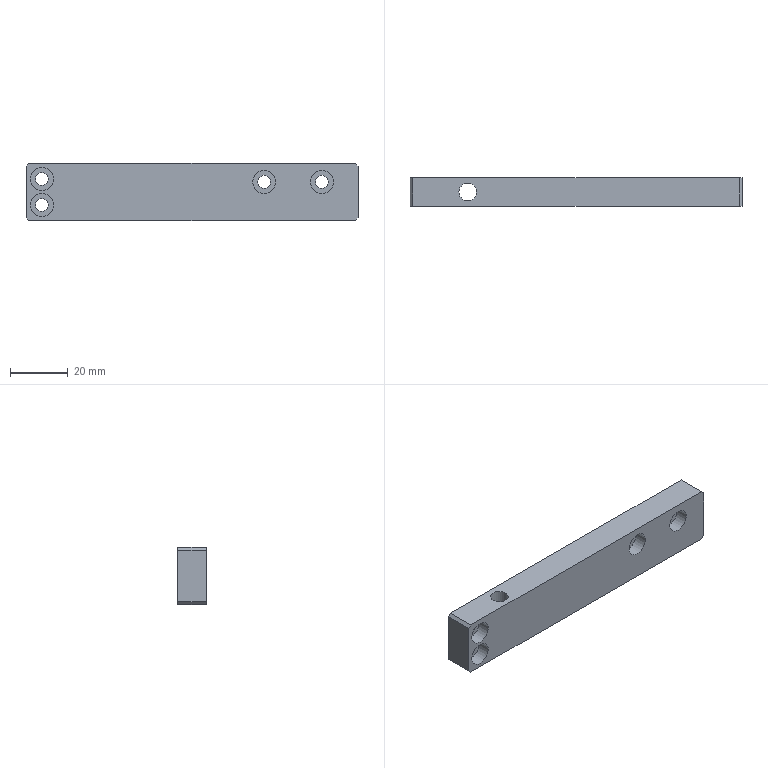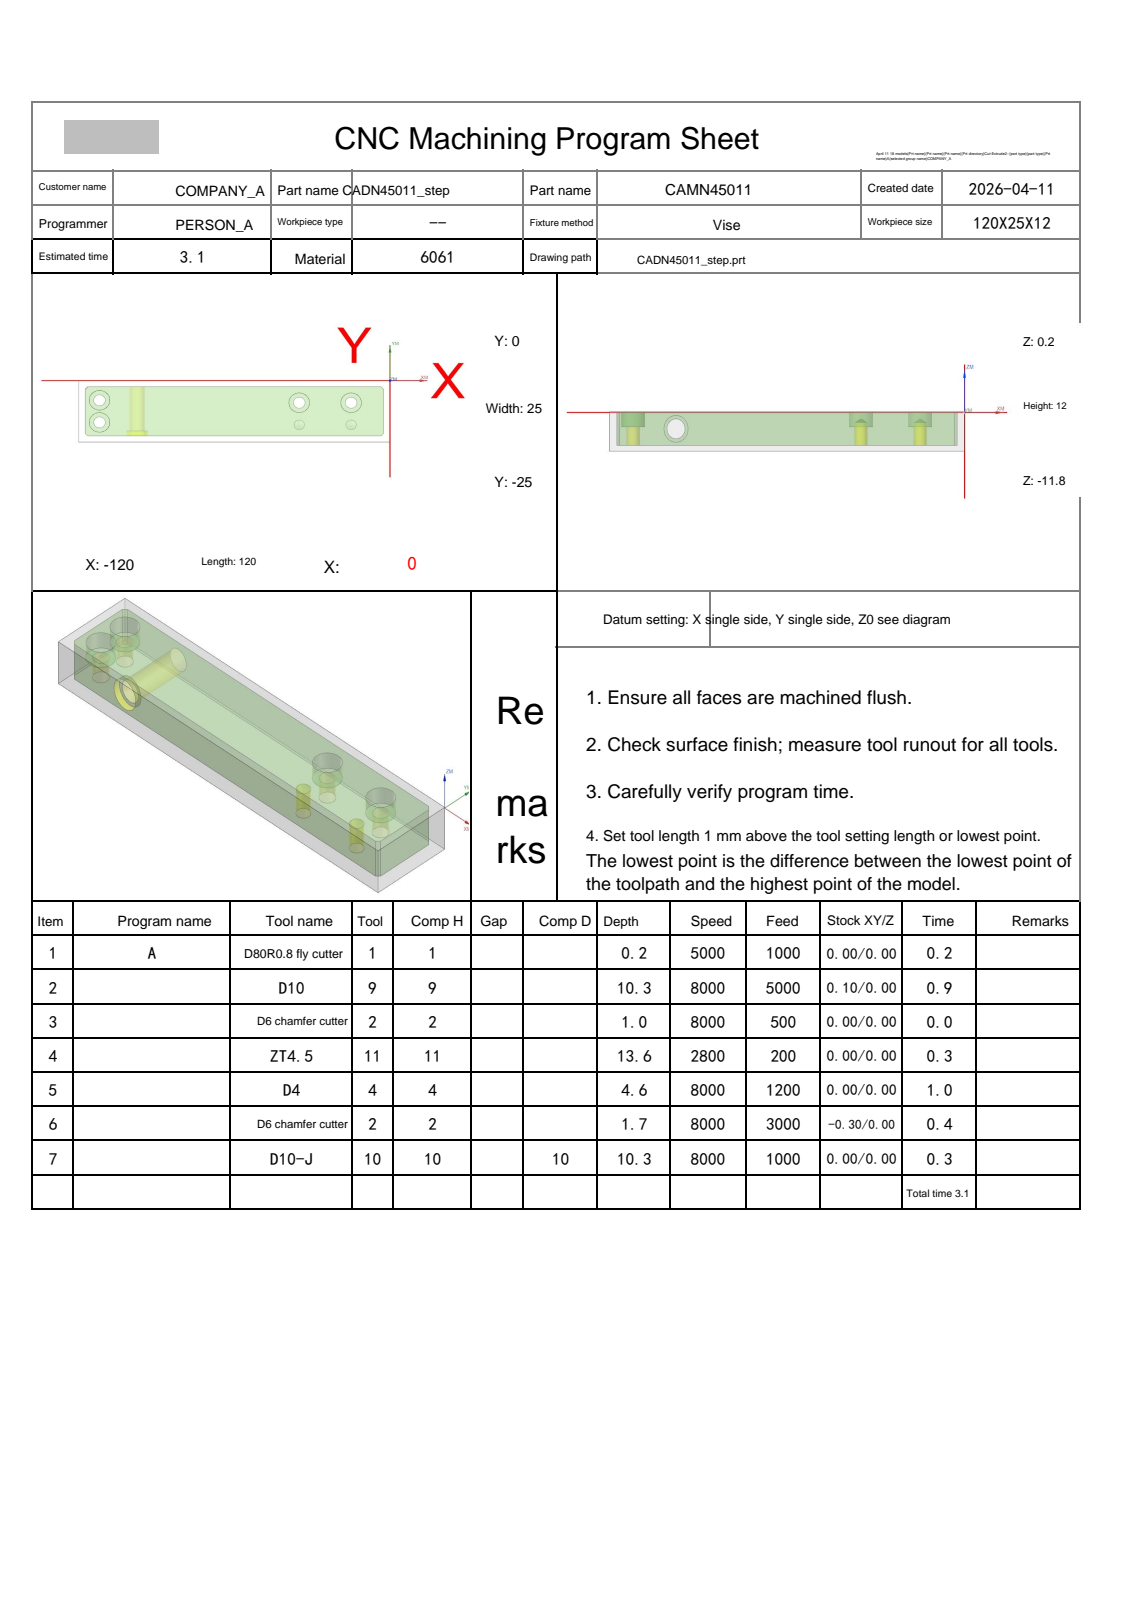NC program | NX | posted by the shop | part box 115 x 10 x 20 mm
Whole program:
%
O0001
(Machine time: 4.57 MIN)
(===Total Tool:6===)
(T1=D80R0.8 fly cutter D=80.  R=0.8  D-  H01 Z=0.    )
(T9=D10     D=10.  R=0.   D-  H09 Z=-10.1 )
(T2=D6 chamfer cutter   D=6.   R=0.   D-  H02 Z=-1.5  )
(T11=ZT4.5  D=4.5  DR_a=118 D-  H11 Z=-13.35)
(T4=D4      D=4.   R=0.   D4  H04 Z=-4.4  )
(T10=D10-J  D=10.  R=0.   D10 H10 Z=-10.1 )
G80 G90 G17 G49 G40
G91 G28 Z0
M01
N1 T01 M06
(D80R0.8 fly cutter  D=80. R=0.8 H=01 ce=0.00 di=0.00)
G00 G90 G54 X42.5 Y-12.5 M03 S5000
G43 H01 Z20.
M08
Z2.
G01 Z0.0 F1000.
X37.5
X-157.5
X-162.5
Z2.
G00 Z20.
G91 G28 Z0.0
M05
M09
G91 G28 Z0.0
M01
N2 T09 M06
(D10  D=10. R=0. H=09 ce=0.10 di=0.00)
G00 G90 G54 X-60. Y2.6 M03 S8000
G43 H09 Z20.
M08
Z.5
G01 X-3.5 Z.357 F5000.
G02 X.106 Y1.106 Z.347 I0.0 J-5.1
G01 X1.106 Y.106 Z.344
G02 X2.6 Y-3.5 Z.333 I-3.606 J-3.606
G01 Y-21.5 Z.288
G02 X1.106 Y-25.106 Z.278 I-5.1 J0.0
G01 X.106 Y-26.106 Z.274
G02 X-3.5 Y-27.6 Z.264 I-3.606 J3.606
G01 X-116.5 Z-.021
G02 X-120.106 Y-26.106 Z-.031 I0.0 J5.1
G01 X-121.106 Y-25.106 Z-.035
G02 X-122.6 Y-21.5 Z-.045 I3.606 J3.606
G01 Y-3.5 Z-.091
G02 X-121.106 Y.106 Z-.101 I5.1 J0.0
G01 X-120.106 Y1.106 Z-.104
G02 X-116.5 Y2.6 Z-.114 I3.606 J-3.606
G01 X-3.5 Z-.4
G02 X.106 Y1.106 Z-.41 I0.0 J-5.1
G01 X1.106 Y.106 Z-.414
G02 X2.6 Y-3.5 Z-.424 I-3.606 J-3.606
G01 Y-21.5 Z-.469
G02 X1.106 Y-25.106 Z-.479 I-5.1 J0.0
G01 X.106 Y-26.106 Z-.483
G02 X-3.5 Y-27.6 Z-.493 I-3.606 J3.606
G01 X-116.5 Z-.778
G02 X-120.106 Y-26.106 Z-.789 I0.0 J5.1
G01 X-121.106 Y-25.106 Z-.792
G02 X-122.6 Y-21.5 Z-.802 I3.606 J3.606
G01 Y-3.5 Z-.848
G02 X-121.106 Y.106 Z-.858 I5.1 J0.0
G01 X-120.106 Y1.106 Z-.861
G02 X-116.5 Y2.6 Z-.872 I3.606 J-3.606
G01 X-3.5 Z-1.157
G02 X.106 Y1.106 Z-1.167 I0.0 J-5.1
G01 X1.106 Y.106 Z-1.171
G02 X2.6 Y-3.5 Z-1.181 I-3.606 J-3.606
G01 Y-21.5 Z-1.226
G02 X1.106 Y-25.106 Z-1.236 I-5.1 J0.0
G01 X.106 Y-26.106 Z-1.24
G02 X-3.5 Y-27.6 Z-1.25 I-3.606 J3.606
G01 X-116.5 Z-1.536
G02 X-120.106 Y-26.106 Z-1.546 I0.0 J5.1
G01 X-121.106 Y-25.106 Z-1.549
G02 X-122.6 Y-21.5 Z-1.559 I3.606 J3.606
G01 Y-3.5 Z-1.605
G02 X-121.106 Y.106 Z-1.615 I5.1 J0.0
G01 X-120.106 Y1.106 Z-1.619
G02 X-116.5 Y2.6 Z-1.629 I3.606 J-3.606
G01 X-3.5 Z-1.914
G02 X.106 Y1.106 Z-1.924 I0.0 J-5.1
G01 X1.106 Y.106 Z-1.928
G02 X2.6 Y-3.5 Z-1.938 I-3.606 J-3.606
G01 Y-21.5 Z-1.983
G02 X1.106 Y-25.106 Z-1.994 I-5.1 J0.0
G01 X.106 Y-26.106 Z-1.997
G02 X-3.5 Y-27.6 Z-2.007 I-3.606 J3.606
G01 X-116.5 Z-2.293
G02 X-120.106 Y-26.106 Z-2.303 I0.0 J5.1
G01 X-121.106 Y-25.106 Z-2.306
G02 X-122.6 Y-21.5 Z-2.317 I3.606 J3.606
G01 Y-3.5 Z-2.362
G02 X-121.106 Y.106 Z-2.372 I5.1 J0.0
G01 X-120.106 Y1.106 Z-2.376
G02 X-116.5 Y2.6 Z-2.386 I3.606 J-3.606
G01 X-3.5 Z-2.671
G02 X.106 Y1.106 Z-2.681 I0.0 J-5.1
G01 X1.106 Y.106 Z-2.685
G02 X2.6 Y-3.5 Z-2.695 I-3.606 J-3.606
G01 Y-21.5 Z-2.741
G02 X1.106 Y-25.106 Z-2.751 I-5.1 J0.0
G01 X.106 Y-26.106 Z-2.754
G02 X-3.5 Y-27.6 Z-2.764 I-3.606 J3.606
G01 X-116.5 Z-3.05
G02 X-120.106 Y-26.106 Z-3.06 I0.0 J5.1
G01 X-121.106 Y-25.106 Z-3.064
G02 X-122.6 Y-21.5 Z-3.074 I3.606 J3.606
G01 Y-3.5 Z-3.119
G02 X-121.106 Y.106 Z-3.129 I5.1 J0.0
G01 X-120.106 Y1.106 Z-3.133
G02 X-116.5 Y2.6 Z-3.143 I3.606 J-3.606
G01 X-3.5 Z-3.428
G02 X.106 Y1.106 Z-3.439 I0.0 J-5.1
G01 X1.106 Y.106 Z-3.442
G02 X2.6 Y-3.5 Z-3.452 I-3.606 J-3.606
G01 Y-21.5 Z-3.498
G02 X1.106 Y-25.106 Z-3.508 I-5.1 J0.0
G01 X.106 Y-26.106 Z-3.511
G02 X-3.5 Y-27.6 Z-3.522 I-3.606 J3.606
G01 X-116.5 Z-3.807
G02 X-120.106 Y-26.106 Z-3.817 I0.0 J5.1
G01 X-121.106 Y-25.106 Z-3.821
G02 X-122.6 Y-21.5 Z-3.831 I3.606 J3.606
G01 Y-3.5 Z-3.876
G02 X-121.106 Y.106 Z-3.886 I5.1 J0.0
G01 X-120.106 Y1.106 Z-3.89
G02 X-116.5 Y2.6 Z-3.9 I3.606 J-3.606
G01 X-3.5 Z-4.186
G02 X.106 Y1.106 Z-4.196 I0.0 J-5.1
G01 X1.106 Y.106 Z-4.199
G02 X2.6 Y-3.5 Z-4.209 I-3.606 J-3.606
G01 Y-21.5 Z-4.255
G02 X1.106 Y-25.106 Z-4.265 I-5.1 J0.0
G01 X.106 Y-26.106 Z-4.269
G02 X-3.5 Y-27.6 Z-4.279 I-3.606 J3.606
G01 X-116.5 Z-4.564
G02 X-120.106 Y-26.106 Z-4.574 I0.0 J5.1
G01 X-121.106 Y-25.106 Z-4.578
G02 X-122.6 Y-21.5 Z-4.588 I3.606 J3.606
G01 Y-3.5 Z-4.633
G02 X-121.106 Y.106 Z-4.644 I5.1 J0.0
G01 X-120.106 Y1.106 Z-4.647
G02 X-116.5 Y2.6 Z-4.657 I3.606 J-3.606
G01 X-3.5 Z-4.943
G02 X.106 Y1.106 Z-4.953 I0.0 J-5.1
G01 X1.106 Y.106 Z-4.956
G02 X2.6 Y-3.5 Z-4.967 I-3.606 J-3.606
G01 Y-21.5 Z-5.012
G02 X1.106 Y-25.106 Z-5.022 I-5.1 J0.0
G01 X.106 Y-26.106 Z-5.026
G02 X-3.5 Y-27.6 Z-5.036 I-3.606 J3.606
G01 X-116.5 Z-5.321
G02 X-120.106 Y-26.106 Z-5.331 I0.0 J5.1
G01 X-121.106 Y-25.106 Z-5.335
G02 X-122.6 Y-21.5 Z-5.345 I3.606 J3.606
G01 Y-3.5 Z-5.391
G02 X-121.106 Y.106 Z-5.401 I5.1 J0.0
G01 X-120.106 Y1.106 Z-5.404
G02 X-116.5 Y2.6 Z-5.414 I3.606 J-3.606
G01 X-3.5 Z-5.7
G02 X.106 Y1.106 Z-5.71 I0.0 J-5.1
G01 X1.106 Y.106 Z-5.714
G02 X2.6 Y-3.5 Z-5.724 I-3.606 J-3.606
G01 Y-21.5 Z-5.769
G02 X1.106 Y-25.106 Z-5.779 I-5.1 J0.0
G01 X.106 Y-26.106 Z-5.783
G02 X-3.5 Y-27.6 Z-5.793 I-3.606 J3.606
G01 X-116.5 Z-6.078
G02 X-120.106 Y-26.106 Z-6.089 I0.0 J5.1
G01 X-121.106 Y-25.106 Z-6.092
G02 X-122.6 Y-21.5 Z-6.102 I3.606 J3.606
G01 Y-3.5 Z-6.148
G02 X-121.106 Y.106 Z-6.158 I5.1 J0.0
G01 X-120.106 Y1.106 Z-6.161
G02 X-116.5 Y2.6 Z-6.172 I3.606 J-3.606
G01 X-3.5 Z-6.457
G02 X.106 Y1.106 Z-6.467 I0.0 J-5.1
G01 X1.106 Y.106 Z-6.471
G02 X2.6 Y-3.5 Z-6.481 I-3.606 J-3.606
G01 Y-21.5 Z-6.526
G02 X1.106 Y-25.106 Z-6.536 I-5.1 J0.0
G01 X.106 Y-26.106 Z-6.54
G02 X-3.5 Y-27.6 Z-6.55 I-3.606 J3.606
G01 X-116.5 Z-6.836
G02 X-120.106 Y-26.106 Z-6.846 I0.0 J5.1
G01 X-121.106 Y-25.106 Z-6.849
G02 X-122.6 Y-21.5 Z-6.859 I3.606 J3.606
G01 Y-3.5 Z-6.905
G02 X-121.106 Y.106 Z-6.915 I5.1 J0.0
G01 X-120.106 Y1.106 Z-6.919
G02 X-116.5 Y2.6 Z-6.929 I3.606 J-3.606
G01 X-3.5 Z-7.214
G02 X.106 Y1.106 Z-7.224 I0.0 J-5.1
G01 X1.106 Y.106 Z-7.228
G02 X2.6 Y-3.5 Z-7.238 I-3.606 J-3.606
G01 Y-21.5 Z-7.283
G02 X1.106 Y-25.106 Z-7.294 I-5.1 J0.0
G01 X.106 Y-26.106 Z-7.297
G02 X-3.5 Y-27.6 Z-7.307 I-3.606 J3.606
G01 X-116.5 Z-7.593
G02 X-120.106 Y-26.106 Z-7.603 I0.0 J5.1
G01 X-121.106 Y-25.106 Z-7.606
G02 X-122.6 Y-21.5 Z-7.617 I3.606 J3.606
G01 Y-3.5 Z-7.662
G02 X-121.106 Y.106 Z-7.672 I5.1 J0.0
G01 X-120.106 Y1.106 Z-7.676
G02 X-116.5 Y2.6 Z-7.686 I3.606 J-3.606
G01 X-3.5 Z-7.971
G02 X.106 Y1.106 Z-7.981 I0.0 J-5.1
G01 X1.106 Y.106 Z-7.985
G02 X2.6 Y-3.5 Z-7.995 I-3.606 J-3.606
G01 Y-21.5 Z-8.041
G02 X1.106 Y-25.106 Z-8.051 I-5.1 J0.0
G01 X.106 Y-26.106 Z-8.054
G02 X-3.5 Y-27.6 Z-8.064 I-3.606 J3.606
G01 X-116.5 Z-8.35
G02 X-120.106 Y-26.106 Z-8.36 I0.0 J5.1
G01 X-121.106 Y-25.106 Z-8.364
G02 X-122.6 Y-21.5 Z-8.374 I3.606 J3.606
G01 Y-3.5 Z-8.419
G02 X-121.106 Y.106 Z-8.429 I5.1 J0.0
G01 X-120.106 Y1.106 Z-8.433
G02 X-116.5 Y2.6 Z-8.443 I3.606 J-3.606
G01 X-3.5 Z-8.728
G02 X.106 Y1.106 Z-8.739 I0.0 J-5.1
G01 X1.106 Y.106 Z-8.742
G02 X2.6 Y-3.5 Z-8.752 I-3.606 J-3.606
G01 Y-21.5 Z-8.798
G02 X1.106 Y-25.106 Z-8.808 I-5.1 J0.0
G01 X.106 Y-26.106 Z-8.811
G02 X-3.5 Y-27.6 Z-8.822 I-3.606 J3.606
G01 X-116.5 Z-9.107
G02 X-120.106 Y-26.106 Z-9.117 I0.0 J5.1
G01 X-121.106 Y-25.106 Z-9.121
G02 X-122.6 Y-21.5 Z-9.131 I3.606 J3.606
G01 Y-3.5 Z-9.176
G02 X-121.106 Y.106 Z-9.186 I5.1 J0.0
G01 X-120.106 Y1.106 Z-9.19
G02 X-116.5 Y2.6 Z-9.2 I3.606 J-3.606
G01 X-3.5 Z-9.486
G02 X.106 Y1.106 Z-9.496 I0.0 J-5.1
G01 X1.106 Y.106 Z-9.499
G02 X2.6 Y-3.5 Z-9.509 I-3.606 J-3.606
G01 Y-21.5 Z-9.555
G02 X1.106 Y-25.106 Z-9.565 I-5.1 J0.0
G01 X.106 Y-26.106 Z-9.569
G02 X-3.5 Y-27.6 Z-9.579 I-3.606 J3.606
G01 X-116.5 Z-9.864
G02 X-120.106 Y-26.106 Z-9.874 I0.0 J5.1
G01 X-121.106 Y-25.106 Z-9.878
G02 X-122.6 Y-21.5 Z-9.888 I3.606 J3.606
G01 Y-3.5 Z-9.933
G02 X-121.106 Y.106 Z-9.944 I5.1 J0.0
G01 X-120.106 Y1.106 Z-9.947
G02 X-116.5 Y2.6 Z-9.957 I3.606 J-3.606
G01 X-60. Z-10.1
X-3.5
G02 X.106 Y1.106 I0.0 J-5.1
G01 X1.106 Y.106
G02 X2.6 Y-3.5 I-3.606 J-3.606
G01 Y-21.5
G02 X1.106 Y-25.106 I-5.1 J0.0
G01 X.106 Y-26.106
G02 X-3.5 Y-27.6 I-3.606 J3.606
G01 X-116.5
G02 X-120.106 Y-26.106 I0.0 J5.1
G01 X-121.106 Y-25.106
G02 X-122.6 Y-21.5 I3.606 J3.606
G01 Y-3.5
G02 X-121.106 Y.106 I5.1 J0.0
G01 X-120.106 Y1.106
G02 X-116.5 Y2.6 I3.606 J-3.606
G01 X-60.
X-59.5
Z-9.1
G00 Z20.
G91 G28 Z0.0
M05
M09
G91 G28 Z0.0
M01
N3 T02 M06
(D6 chamfer cutter  D=6. R=0. H=02 ce=0.00 di=0.00)
G00 G90 G54 X-112. Y-17. M03 S8000
G43 H02 Z20.
M08
G98 G81 X-112. Y-17. Z-.8 R1. F500.
Y-8.
X-35. Y-9.
X-15.
G80
G00 Z20.
G91 G28 Z0.0
M05
M09
G91 G28 Z0.0
M01
N4 T11 M06
(ZT4.5 D=4.5 DR_a=118 H=11)
G00 G90 G54 X-112. Y-17. M03 S2800
G43 H11 Z20.
M08
G98 G83 X-112. Y-17. Z-13.352 R1. F200. Q2.
Y-8.
X-35. Y-9.
X-15.
G80
G00 Z20.
G91 G28 Z0.0
M05
M09
G91 G28 Z0.0
M01
N5 T04 M06
(D4  D=4. R=0. H=04 ce=0.10 di=0.00)
G00 G90 G54 X-112. Y-8. M03 S8000
G43 H04 Z20.
M08
Z.5
G03 X-111.05 Y-8.95 I.95 J0.0 F1200.
X-110.1 Y-8. I0.0 J.95
X-110.1 Y-8. Z.2 I-1.9 J0.0
X-110.1 Y-8. Z-.1 I-1.9 J0.0
X-110.1 Y-8. Z-.4 I-1.9 J0.0
X-110.1 Y-8. Z-.7 I-1.9 J0.0
X-110.1 Y-8. Z-1. I-1.9 J0.0
X-110.1 Y-8. Z-1.3 I-1.9 J0.0
X-110.1 Y-8. Z-1.6 I-1.9 J0.0
X-110.1 Y-8. Z-1.9 I-1.9 J0.0
X-110.1 Y-8. Z-2.2 I-1.9 J0.0
X-110.1 Y-8. Z-2.5 I-1.9 J0.0
X-110.1 Y-8. Z-2.8 I-1.9 J0.0
X-110.1 Y-8. Z-3.1 I-1.9 J0.0
X-110.1 Y-8. Z-3.4 I-1.9 J0.0
X-110.1 Y-8. Z-3.7 I-1.9 J0.0
X-110.1 Y-8. Z-4. I-1.9 J0.0
X-110.1 Y-8. Z-4.3 I-1.9 J0.0
X-112.95 Y-6.355 Z-4.4 I-1.9 J0.0
X-113.9 Y-8. I.95 J-1.645
X-112. Y-9.9 I1.9 J0.0
X-110.1 Y-8. I0.0 J1.9
X-112. Y-6.1 I-1.9 J0.0
X-112.95 Y-6.355 I0.0 J-1.9
X-113.425 Y-7.177 I.475 J-.823
X-112.475 Y-8.127 I.95 J0.0
X-112. Y-8. I0.0 J.95
G00 Z20.
Y-17.
Z.5
G03 X-111.05 Y-17.95 I.95 J0.0
X-110.1 Y-17. I0.0 J.95
X-110.1 Y-17. Z.2 I-1.9 J0.0
X-110.1 Y-17. Z-.1 I-1.9 J0.0
X-110.1 Y-17. Z-.4 I-1.9 J0.0
X-110.1 Y-17. Z-.7 I-1.9 J0.0
X-110.1 Y-17. Z-1. I-1.9 J0.0
X-110.1 Y-17. Z-1.3 I-1.9 J0.0
X-110.1 Y-17. Z-1.6 I-1.9 J0.0
X-110.1 Y-17. Z-1.9 I-1.9 J0.0
X-110.1 Y-17. Z-2.2 I-1.9 J0.0
X-110.1 Y-17. Z-2.5 I-1.9 J0.0
X-110.1 Y-17. Z-2.8 I-1.9 J0.0
X-110.1 Y-17. Z-3.1 I-1.9 J0.0
X-110.1 Y-17. Z-3.4 I-1.9 J0.0
X-110.1 Y-17. Z-3.7 I-1.9 J0.0
X-110.1 Y-17. Z-4. I-1.9 J0.0
X-110.1 Y-17. Z-4.3 I-1.9 J0.0
X-112.95 Y-15.355 Z-4.4 I-1.9 J0.0
X-113.9 Y-17. I.95 J-1.645
X-112. Y-18.9 I1.9 J0.0
X-110.1 Y-17. I0.0 J1.9
X-112. Y-15.1 I-1.9 J0.0
X-112.95 Y-15.355 I0.0 J-1.9
X-113.425 Y-16.177 I.475 J-.823
X-112.475 Y-17.127 I.95 J0.0
X-112. Y-17. I0.0 J.95
G00 Z20.
X-35. Y-9.
Z.5
G03 X-34.05 Y-9.95 I.95 J0.0
X-33.1 Y-9. I0.0 J.95
X-33.1 Y-9. Z.2 I-1.9 J0.0
X-33.1 Y-9. Z-.1 I-1.9 J0.0
X-33.1 Y-9. Z-.4 I-1.9 J0.0
X-33.1 Y-9. Z-.7 I-1.9 J0.0
X-33.1 Y-9. Z-1. I-1.9 J0.0
X-33.1 Y-9. Z-1.3 I-1.9 J0.0
X-33.1 Y-9. Z-1.6 I-1.9 J0.0
X-33.1 Y-9. Z-1.9 I-1.9 J0.0
X-33.1 Y-9. Z-2.2 I-1.9 J0.0
X-33.1 Y-9. Z-2.5 I-1.9 J0.0
X-33.1 Y-9. Z-2.8 I-1.9 J0.0
X-33.1 Y-9. Z-3.1 I-1.9 J0.0
X-33.1 Y-9. Z-3.4 I-1.9 J0.0
X-33.1 Y-9. Z-3.7 I-1.9 J0.0
X-33.1 Y-9. Z-4. I-1.9 J0.0
X-33.1 Y-9. Z-4.3 I-1.9 J0.0
X-35.95 Y-7.355 Z-4.4 I-1.9 J0.0
X-36.9 Y-9. I.95 J-1.645
X-35. Y-10.9 I1.9 J0.0
X-33.1 Y-9. I0.0 J1.9
X-35. Y-7.1 I-1.9 J0.0
X-35.95 Y-7.355 I0.0 J-1.9
X-36.425 Y-8.177 I.475 J-.823
X-35.475 Y-9.127 I.95 J0.0
X-35. Y-9. I0.0 J.95
G00 Z20.
X-15.
Z.5
G03 X-14.05 Y-9.95 I.95 J0.0
X-13.1 Y-9. I0.0 J.95
X-13.1 Y-9. Z.2 I-1.9 J0.0
X-13.1 Y-9. Z-.1 I-1.9 J0.0
X-13.1 Y-9. Z-.4 I-1.9 J0.0
X-13.1 Y-9. Z-.7 I-1.9 J0.0
X-13.1 Y-9. Z-1. I-1.9 J0.0
X-13.1 Y-9. Z-1.3 I-1.9 J0.0
X-13.1 Y-9. Z-1.6 I-1.9 J0.0
X-13.1 Y-9. Z-1.9 I-1.9 J0.0
X-13.1 Y-9. Z-2.2 I-1.9 J0.0
X-13.1 Y-9. Z-2.5 I-1.9 J0.0
X-13.1 Y-9. Z-2.8 I-1.9 J0.0
X-13.1 Y-9. Z-3.1 I-1.9 J0.0
X-13.1 Y-9. Z-3.4 I-1.9 J0.0
X-13.1 Y-9. Z-3.7 I-1.9 J0.0
X-13.1 Y-9. Z-4. I-1.9 J0.0
X-13.1 Y-9. Z-4.3 I-1.9 J0.0
X-15.95 Y-7.355 Z-4.4 I-1.9 J0.0
X-16.9 Y-9. I.95 J-1.645
X-15. Y-10.9 I1.9 J0.0
X-13.1 Y-9. I0.0 J1.9
X-15. Y-7.1 I-1.9 J0.0
X-15.95 Y-7.355 I0.0 J-1.9
X-16.425 Y-8.177 I.475 J-.823
X-15.475 Y-9.127 I.95 J0.0
X-15. Y-9. I0.0 J.95
G00 Z20.
G00 G90 X-112. Y-8. M03 S8000
Z20.
Z.5
G41 D04
G01 X-111.96 Y-8.196 F500.
G03 X-110.99 Y-8.99 I.97 J.196
X-110. Y-8. I0.0 J.99
X-110.016 Y-8.251 Z-4.4 I-2. J0.0
X-110. Y-8. I-1.984 J.251
X-112. Y-6. I-2. J0.0
X-114. Y-8. I0.0 J-2.
X-112. Y-10. I2. J0.0
X-110.016 Y-8.251 I0.0 J2.
G01 X-110.008 Y-8.127
G03 X-110.998 Y-7.137 I-.99 J0.0
X-111.936 Y-7.81 I0.0 J-.99
G01 G40 X-112. Y-8.
G00 Z20.
Y-17.
Z.5
G41 D04
G01 X-111.96 Y-17.196
G03 X-110.99 Y-17.99 I.97 J.196
X-110. Y-17. I0.0 J.99
X-110.016 Y-17.251 Z-4.4 I-2. J0.0
X-110. Y-17. I-1.984 J.251
X-112. Y-15. I-2. J0.0
X-114. Y-17. I0.0 J-2.
X-112. Y-19. I2. J0.0
X-110.016 Y-17.251 I0.0 J2.
G01 X-110.008 Y-17.127
G03 X-110.998 Y-16.137 I-.99 J0.0
X-111.936 Y-16.81 I0.0 J-.99
G01 G40 X-112. Y-17.
G00 Z20.
X-35. Y-9.
Z.5
G41 D04
G01 X-34.96 Y-9.196
G03 X-33.99 Y-9.99 I.97 J.196
X-33. Y-9. I0.0 J.99
X-33.016 Y-9.251 Z-4.4 I-2. J0.0
X-33. Y-9. I-1.984 J.251
X-35. Y-7. I-2. J0.0
X-37. Y-9. I0.0 J-2.
X-35. Y-11. I2. J0.0
X-33.016 Y-9.251 I0.0 J2.
G01 X-33.008 Y-9.127
G03 X-33.998 Y-8.137 I-.99 J0.0
X-34.936 Y-8.81 I0.0 J-.99
G01 G40 X-35. Y-9.
G00 Z20.
X-15.
Z.5
G41 D04
G01 X-14.96 Y-9.196
G03 X-13.99 Y-9.99 I.97 J.196
X-13. Y-9. I0.0 J.99
X-13.016 Y-9.251 Z-4.4 I-2. J0.0
X-13. Y-9. I-1.984 J.251
X-15. Y-7. I-2. J0.0
X-17. Y-9. I0.0 J-2.
X-15. Y-11. I2. J0.0
X-13.016 Y-9.251 I0.0 J2.
G01 X-13.008 Y-9.127
G03 X-13.998 Y-8.137 I-.99 J0.0
X-14.936 Y-8.81 I0.0 J-.99
G01 G40 X-15. Y-9.
G00 Z20.
G91 G28 Z0.0
M05
M09
G91 G28 Z0.0
M01
N6 T02 M06
(D6 chamfer cutter  D=6. R=0. H=02 ce=0.00 di=0.00)
G00 G90 G54 X-60.25 Y-.372 M03 S8000
G43 H02 Z20.
M08
Z2.099
G01 Z-1.5 F3000.
G03 X-60.33 Y-.672 I.52 J-.3
X-60.03 Y-1.192 I.6 J0.0
G01 X-60. Y-1.2
X-3.5
X-3.246 Y-1.225
X-3.003 Y-1.299
X-2.778 Y-1.419
X-2.581 Y-1.581
X-1.581 Y-2.581
X-1.419 Y-2.778
X-1.299 Y-3.003
X-1.225 Y-3.246
X-1.2 Y-3.5
Y-21.5
X-1.225 Y-21.754
X-1.299 Y-21.997
X-1.419 Y-22.222
X-1.581 Y-22.419
X-2.581 Y-23.419
X-2.778 Y-23.581
X-3.003 Y-23.701
X-3.246 Y-23.775
X-3.5 Y-23.8
X-116.5
X-116.754 Y-23.775
X-116.997 Y-23.701
X-117.222 Y-23.581
X-117.419 Y-23.419
X-118.419 Y-22.419
X-118.581 Y-22.222
X-118.701 Y-21.997
X-118.775 Y-21.754
X-118.8 Y-21.5
Y-3.5
X-118.775 Y-3.246
X-118.701 Y-3.003
X-118.581 Y-2.778
X-118.419 Y-2.581
X-117.419 Y-1.581
X-117.222 Y-1.419
X-116.997 Y-1.299
X-116.754 Y-1.225
X-116.5 Y-1.2
X-60.
X-59.97 Y-1.192
G03 X-59.67 Y-.672 I-.3 J.52
X-59.75 Y-.372 I-.6 J0.0
G01 Z2.099
G00 Z20.
G00 G90 X-111.253 Y-20.212 M03 S8000
Z20.
Z2.5
G01 X-111.038 Y-20.16 Z2.42 F500.
X-110.672 Y-20.024 Z2.278
X-110.325 Y-19.847 Z2.136
X-110.001 Y-19.629 Z1.994
X-109.705 Y-19.375 Z1.852
X-109.441 Y-19.088 Z1.71
X-109.212 Y-18.772 Z1.568
X-109.072 Y-18.528 Z1.465
X-108.912 Y-18.172 Z1.323
X-108.795 Y-17.8 Z1.181
X-108.723 Y-17.416 Z1.039
X-108.697 Y-17.027 Z.897
X-108.717 Y-16.638 Z.755
X-108.783 Y-16.253 Z.613
X-108.893 Y-15.879 Z.471
X-109.047 Y-15.52 Z.329
X-109.242 Y-15.182 Z.187
X-109.476 Y-14.87 Z.045
X-109.744 Y-14.587 Z-.097
X-110.045 Y-14.338 Z-.239
X-110.372 Y-14.126 Z-.381
X-110.722 Y-13.954 Z-.523
X-111.09 Y-13.825 Z-.665
X-111.471 Y-13.74 Z-.807
X-111.859 Y-13.7 Z-.949
X-112. Z-1.
G03 X-115.3 Y-17. I0.0 J-3.3
X-112. Y-20.3 I3.3 J0.0
X-108.7 Y-17. I0.0 J3.3
X-112. Y-13.7 I-3.3 J0.0
X-112.498 Y-13.738 I0.0 J-3.3
G01 Z1.5
G00 Z20.
X-111.253 Y-11.212
Z2.5
G01 X-111.038 Y-11.16 Z2.42
X-110.672 Y-11.024 Z2.278
X-110.325 Y-10.847 Z2.136
X-110.001 Y-10.629 Z1.994
X-109.705 Y-10.375 Z1.852
X-109.441 Y-10.088 Z1.71
X-109.212 Y-9.772 Z1.568
X-109.072 Y-9.528 Z1.465
X-108.912 Y-9.172 Z1.323
X-108.795 Y-8.8 Z1.181
X-108.723 Y-8.416 Z1.039
X-108.697 Y-8.027 Z.897
X-108.717 Y-7.638 Z.755
X-108.783 Y-7.253 Z.613
X-108.893 Y-6.879 Z.471
X-109.047 Y-6.52 Z.329
X-109.242 Y-6.182 Z.187
X-109.476 Y-5.87 Z.045
X-109.744 Y-5.587 Z-.097
X-110.045 Y-5.338 Z-.239
X-110.372 Y-5.126 Z-.381
X-110.722 Y-4.954 Z-.523
X-111.09 Y-4.825 Z-.665
X-111.471 Y-4.74 Z-.807
X-111.859 Y-4.7 Z-.949
X-112. Z-1.
G03 X-115.3 Y-8. I0.0 J-3.3
X-112. Y-11.3 I3.3 J0.0
X-108.7 Y-8. I0.0 J3.3
X-112. Y-4.7 I-3.3 J0.0
X-112.498 Y-4.738 I0.0 J-3.3
G01 Z1.5
G00 Z20.
X-34.253 Y-12.212
Z2.5
G01 X-34.038 Y-12.16 Z2.42
X-33.672 Y-12.024 Z2.278
X-33.325 Y-11.847 Z2.136
X-33.001 Y-11.629 Z1.994
X-32.705 Y-11.375 Z1.852
X-32.441 Y-11.088 Z1.71
X-32.212 Y-10.772 Z1.568
X-32.072 Y-10.528 Z1.465
X-31.912 Y-10.172 Z1.323
X-31.795 Y-9.8 Z1.181
X-31.723 Y-9.416 Z1.039
X-31.697 Y-9.027 Z.897
X-31.717 Y-8.638 Z.755
X-31.783 Y-8.253 Z.613
X-31.893 Y-7.879 Z.471
X-32.047 Y-7.52 Z.329
X-32.242 Y-7.182 Z.187
X-32.476 Y-6.87 Z.045
X-32.744 Y-6.587 Z-.097
X-33.045 Y-6.338 Z-.239
X-33.372 Y-6.126 Z-.381
X-33.722 Y-5.954 Z-.523
X-34.09 Y-5.825 Z-.665
X-34.471 Y-5.74 Z-.807
X-34.859 Y-5.7 Z-.949
X-35. Z-1.
G03 X-38.3 Y-9. I0.0 J-3.3
X-35. Y-12.3 I3.3 J0.0
X-31.7 Y-9. I0.0 J3.3
X-35. Y-5.7 I-3.3 J0.0
X-35.498 Y-5.738 I0.0 J-3.3
G01 Z1.5
G00 Z20.
X-14.253 Y-12.212
Z2.5
G01 X-14.038 Y-12.16 Z2.42
X-13.672 Y-12.024 Z2.278
X-13.325 Y-11.847 Z2.136
X-13.001 Y-11.629 Z1.994
X-12.705 Y-11.375 Z1.852
X-12.441 Y-11.088 Z1.71
X-12.212 Y-10.772 Z1.568
X-12.072 Y-10.528 Z1.465
X-11.912 Y-10.172 Z1.323
X-11.795 Y-9.8 Z1.181
X-11.723 Y-9.416 Z1.039
X-11.697 Y-9.027 Z.897
X-11.717 Y-8.638 Z.755
X-11.783 Y-8.253 Z.613
X-11.893 Y-7.879 Z.471
X-12.047 Y-7.52 Z.329
X-12.242 Y-7.182 Z.187
X-12.476 Y-6.87 Z.045
X-12.744 Y-6.587 Z-.097
X-13.045 Y-6.338 Z-.239
X-13.372 Y-6.126 Z-.381
X-13.722 Y-5.954 Z-.523
X-14.09 Y-5.825 Z-.665
X-14.471 Y-5.74 Z-.807
X-14.859 Y-5.7 Z-.949
X-15. Z-1.
G03 X-18.3 Y-9. I0.0 J-3.3
X-15. Y-12.3 I3.3 J0.0
X-11.7 Y-9. I0.0 J3.3
X-15. Y-5.7 I-3.3 J0.0
X-15.498 Y-5.738 I0.0 J-3.3
G01 Z1.5
G00 Z20.
G91 G28 Z0.0
M05
M09
G91 G28 Z0.0
M01
N7 T10 M06
(D10-J  D=10. R=0. H=10 ce=0.00 di=0.00)
G00 G90 G54 X-117.513 Y3.616 M03 S8000
G43 H10 Z20.
M08
Z-9.6
G01 Z-10.1 F1000.
G41 D10
X-117.497 Y3.417
G03 X-116.5 Y2.5 I.997 J.083
G01 X-3.5
G02 X.036 Y1.036 I0.0 J-5.
G01 X1.036 Y.036
G02 X2.5 Y-3.5 I-3.536 J-3.536
G01 Y-21.5
G02 X1.036 Y-25.036 I-5. J0.0
G01 X.036 Y-26.036
G02 X-3.5 Y-27.5 I-3.536 J3.536
G01 X-116.5
G02 X-120.036 Y-26.036 I0.0 J5.
G01 X-121.036 Y-25.036
G02 X-122.5 Y-21.5 I3.536 J3.536
G01 Y-3.5
G02 X-121.036 Y.036 I5. J0.0
G01 X-120.036 Y1.036
G02 X-116.5 Y2.5 I3.536 J-3.536
G01 X-116.
G03 X-115. Y3.5 I0.0 J1.
G01 G40 Y3.7
Z-9.6
G00 Z20.
M05
M09
G91 G28 Z0.0
G91 G28 Y0.0
M30
%